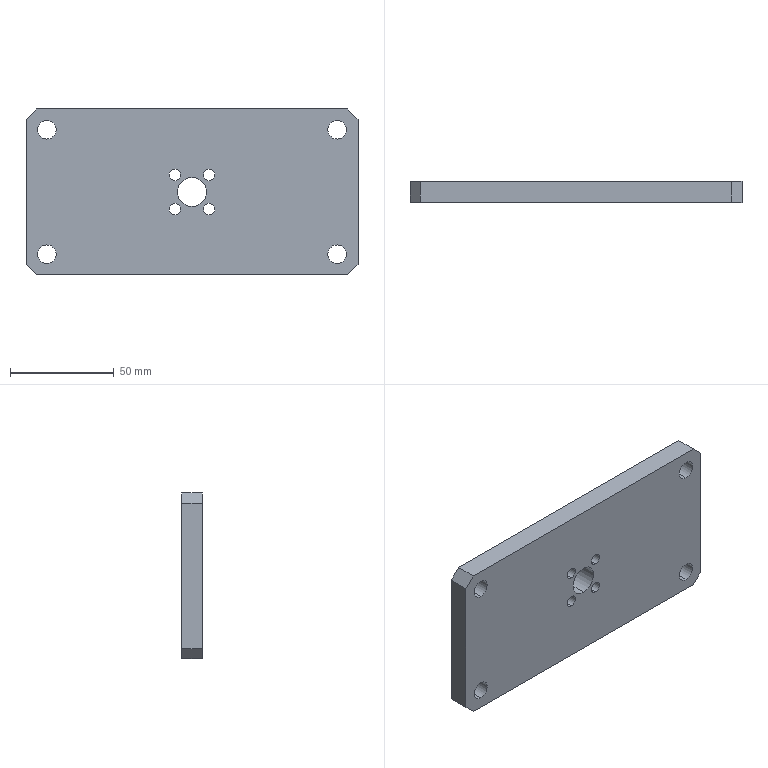Part | STEP file | 0229_203_Plate | 1 solid | 28 faces | box 160 x 10 x 80 mm | volume 122466 mm3 | cylinder 18 | plane 10 | commonest cylinder face diameters 5.5 x8 9 x8 14 x2